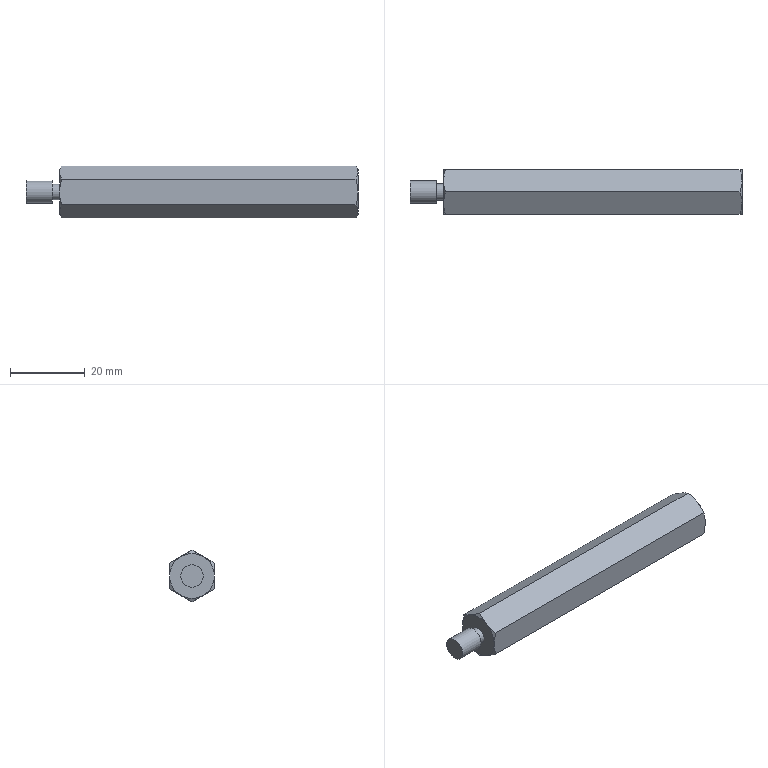Part | NX | features 5003_317_C-PLSBWRK12-80 2 | 1 solid | 26 faces | box 89 x 12 x 13.856 mm | volume 9868 mm3 | cone 13 | plane 10 | cylinder 3 | commonest cylinder face diameters 4.3 x1 4.917 x1 6 x1
STEP:
#1=CARTESIAN_POINT('',(218.525,69.,-97.));
#2=VERTEX_POINT('',#1);
#3=CARTESIAN_POINT('',(218.525,66.,-91.804));
#4=VERTEX_POINT('',#3);
#5=CARTESIAN_POINT('',(218.525,63.,-97.));
#6=DIRECTION('',(1.,0.,0.));
#7=DIRECTION('',(0.,1.,0.));
#8=AXIS2_PLACEMENT_3D('',#5,#6,#7);
#9=CIRCLE('',#8,6.);
#10=EDGE_CURVE('',#2,#4,#9,.T.);
#11=ORIENTED_EDGE('',*,*,#10,.F.);
#12=CARTESIAN_POINT('',(218.525,66.,-102.196));
#13=VERTEX_POINT('',#12);
#14=CARTESIAN_POINT('',(218.525,63.,-97.));
#15=DIRECTION('',(1.,0.,0.));
#16=DIRECTION('',(0.,1.,0.));
#17=AXIS2_PLACEMENT_3D('',#14,#15,#16);
#18=CIRCLE('',#17,6.);
#19=EDGE_CURVE('',#13,#2,#18,.T.);
#20=ORIENTED_EDGE('',*,*,#19,.F.);
#21=CARTESIAN_POINT('',(218.525,60.,-102.196));
#22=VERTEX_POINT('',#21);
#23=CARTESIAN_POINT('',(218.525,63.,-97.));
#24=DIRECTION('',(1.,0.,0.));
#25=DIRECTION('',(0.,1.,0.));
#26=AXIS2_PLACEMENT_3D('',#23,#24,#25);
#27=CIRCLE('',#26,6.);
#28=EDGE_CURVE('',#22,#13,#27,.T.);
#29=ORIENTED_EDGE('',*,*,#28,.F.);
#30=CARTESIAN_POINT('',(218.525,57.,-97.));
#31=VERTEX_POINT('',#30);
#32=CARTESIAN_POINT('',(218.525,63.,-97.));
#33=DIRECTION('',(1.,0.,0.));
#34=DIRECTION('',(0.,1.,0.));
#35=AXIS2_PLACEMENT_3D('',#32,#33,#34);
#36=CIRCLE('',#35,6.);
#37=EDGE_CURVE('',#31,#22,#36,.T.);
#38=ORIENTED_EDGE('',*,*,#37,.F.);
#39=CARTESIAN_POINT('',(218.525,60.,-91.804));
#40=VERTEX_POINT('',#39);
#41=CARTESIAN_POINT('',(218.525,63.,-97.));
#42=DIRECTION('',(-1.,0.,0.));
#43=DIRECTION('',(0.,-1.,0.));
#44=AXIS2_PLACEMENT_3D('',#41,#42,#43);
#45=CIRCLE('',#44,6.);
#46=EDGE_CURVE('',#31,#40,#45,.T.);
#47=ORIENTED_EDGE('',*,*,#46,.T.);
#48=CARTESIAN_POINT('',(218.525,63.,-97.));
#49=DIRECTION('',(1.,0.,0.));
#50=DIRECTION('',(0.,1.,0.));
#51=AXIS2_PLACEMENT_3D('',#48,#49,#50);
#52=CIRCLE('',#51,6.);
#53=EDGE_CURVE('',#4,#40,#52,.T.);
#54=ORIENTED_EDGE('',*,*,#53,.F.);
#55=EDGE_LOOP('',(#11,#20,#29,#38,#47,#54));
#56=FACE_BOUND('',#55,.T.);
#57=CARTESIAN_POINT('',(218.525,65.15,-97.));
#58=VERTEX_POINT('',#57);
#59=CARTESIAN_POINT('',(218.525,63.,-97.));
#60=DIRECTION('',(1.,0.,0.));
#61=DIRECTION('',(0.,1.,0.));
#62=AXIS2_PLACEMENT_3D('',#59,#60,#61);
#63=CIRCLE('',#62,2.15);
#64=EDGE_CURVE('',#58,#58,#63,.F.);
#65=ORIENTED_EDGE('',*,*,#64,.F.);
#66=EDGE_LOOP('',(#65));
#67=FACE_BOUND('',#66,.T.);
#68=CARTESIAN_POINT('',(218.525,63.,-97.));
#69=DIRECTION('',(1.,0.,0.));
#70=DIRECTION('',(0.,1.,0.));
#71=AXIS2_PLACEMENT_3D('',#68,#69,#70);
#72=PLANE('',#71);
#73=ADVANCED_FACE('',(#56,#67),#72,.F.);
#74=CARTESIAN_POINT('',(297.989,69.,-100.464));
#75=VERTEX_POINT('',#74);
#76=CARTESIAN_POINT('',(298.525,69.,-97.));
#77=VERTEX_POINT('',#76);
#78=CARTESIAN_POINT('',(297.989,69.,-100.464));
#79=CARTESIAN_POINT('',(298.314,69.,-99.337));
#80=CARTESIAN_POINT('',(298.525,69.,-98.171));
#81=CARTESIAN_POINT('',(298.525,69.,-97.));
#82=B_SPLINE_CURVE_WITH_KNOTS('',3,(#78,#79,#80,#81),.UNSPECIFIED.,.F.,.F.,(4,4),(0.00618,0.009685),.UNSPECIFIED.);
#83=EDGE_CURVE('',#75,#77,#82,.T.);
#84=ORIENTED_EDGE('',*,*,#83,.F.);
#85=CARTESIAN_POINT('',(219.061,69.,-100.464));
#86=VERTEX_POINT('',#85);
#87=CARTESIAN_POINT('',(298.525,69.,-100.464));
#88=DIRECTION('',(-1.,0.,0.));
#89=VECTOR('',#88,1000.);
#90=LINE('',#87,#89);
#91=EDGE_CURVE('',#75,#86,#90,.T.);
#92=ORIENTED_EDGE('',*,*,#91,.T.);
#93=CARTESIAN_POINT('',(219.061,69.,-100.464));
#94=CARTESIAN_POINT('',(218.736,69.,-99.337));
#95=CARTESIAN_POINT('',(218.525,69.,-98.171));
#96=CARTESIAN_POINT('',(218.525,69.,-97.));
#97=B_SPLINE_CURVE_WITH_KNOTS('',3,(#93,#94,#95,#96),.UNSPECIFIED.,.F.,.F.,(4,4),(0.00618,0.009685),.UNSPECIFIED.);
#98=EDGE_CURVE('',#2,#86,#97,.F.);
#99=ORIENTED_EDGE('',*,*,#98,.F.);
#100=CARTESIAN_POINT('',(219.061,69.,-93.536));
#101=VERTEX_POINT('',#100);
#102=CARTESIAN_POINT('',(218.525,69.,-97.));
#103=CARTESIAN_POINT('',(218.525,69.,-95.829));
#104=CARTESIAN_POINT('',(218.738,69.,-94.656));
#105=CARTESIAN_POINT('',(219.061,69.,-93.536));
#106=B_SPLINE_CURVE_WITH_KNOTS('',3,(#102,#103,#104,#105),.UNSPECIFIED.,.F.,.F.,(4,4),(0.009685,0.01319),.UNSPECIFIED.);
#107=EDGE_CURVE('',#101,#2,#106,.F.);
#108=ORIENTED_EDGE('',*,*,#107,.F.);
#109=CARTESIAN_POINT('',(297.989,69.,-93.536));
#110=VERTEX_POINT('',#109);
#111=CARTESIAN_POINT('',(298.525,69.,-93.536));
#112=DIRECTION('',(-1.,0.,0.));
#113=VECTOR('',#112,1000.);
#114=LINE('',#111,#113);
#115=EDGE_CURVE('',#110,#101,#114,.T.);
#116=ORIENTED_EDGE('',*,*,#115,.F.);
#117=CARTESIAN_POINT('',(298.525,69.,-97.));
#118=CARTESIAN_POINT('',(298.525,69.,-95.829));
#119=CARTESIAN_POINT('',(298.312,69.,-94.656));
#120=CARTESIAN_POINT('',(297.989,69.,-93.536));
#121=B_SPLINE_CURVE_WITH_KNOTS('',3,(#117,#118,#119,#120),.UNSPECIFIED.,.F.,.F.,(4,4),(0.009685,0.01319),.UNSPECIFIED.);
#122=EDGE_CURVE('',#77,#110,#121,.T.);
#123=ORIENTED_EDGE('',*,*,#122,.F.);
#124=EDGE_LOOP('',(#84,#92,#99,#108,#116,#123));
#125=FACE_BOUND('',#124,.T.);
#126=CARTESIAN_POINT('',(298.525,69.,-100.464));
#127=DIRECTION('',(0.,-1.,0.));
#128=DIRECTION('',(0.,0.,-1.));
#129=AXIS2_PLACEMENT_3D('',#126,#127,#128);
#130=PLANE('',#129);
#131=ADVANCED_FACE('',(#125),#130,.F.);
#132=CARTESIAN_POINT('',(298.525,66.,-91.804));
#133=VERTEX_POINT('',#132);
#134=CARTESIAN_POINT('',(297.989,69.,-93.536));
#135=CARTESIAN_POINT('',(298.316,68.018,-92.969));
#136=CARTESIAN_POINT('',(298.525,67.022,-92.394));
#137=CARTESIAN_POINT('',(298.525,66.,-91.804));
#138=B_SPLINE_CURVE_WITH_KNOTS('',3,(#134,#135,#136,#137),.UNSPECIFIED.,.F.,.F.,(4,4),(0.000000238,0.003505),.UNSPECIFIED.);
#139=EDGE_CURVE('',#110,#133,#138,.T.);
#140=ORIENTED_EDGE('',*,*,#139,.F.);
#141=ORIENTED_EDGE('',*,*,#115,.T.);
#142=CARTESIAN_POINT('',(218.525,66.,-91.804));
#143=CARTESIAN_POINT('',(218.525,67.018,-92.392));
#144=CARTESIAN_POINT('',(218.735,68.021,-92.971));
#145=CARTESIAN_POINT('',(219.061,69.,-93.536));
#146=B_SPLINE_CURVE_WITH_KNOTS('',3,(#142,#143,#144,#145),.UNSPECIFIED.,.F.,.F.,(4,4),(0.003505,0.006997),.UNSPECIFIED.);
#147=EDGE_CURVE('',#4,#101,#146,.T.);
#148=ORIENTED_EDGE('',*,*,#147,.F.);
#149=CARTESIAN_POINT('',(219.061,63.,-90.072));
#150=VERTEX_POINT('',#149);
#151=CARTESIAN_POINT('',(219.061,63.,-90.072));
#152=CARTESIAN_POINT('',(218.734,63.982,-90.638));
#153=CARTESIAN_POINT('',(218.525,64.978,-91.214));
#154=CARTESIAN_POINT('',(218.525,66.,-91.804));
#155=B_SPLINE_CURVE_WITH_KNOTS('',3,(#151,#152,#153,#154),.UNSPECIFIED.,.F.,.F.,(4,4),(0.000000238,0.003505),.UNSPECIFIED.);
#156=EDGE_CURVE('',#150,#4,#155,.T.);
#157=ORIENTED_EDGE('',*,*,#156,.F.);
#158=CARTESIAN_POINT('',(297.989,63.,-90.072));
#159=VERTEX_POINT('',#158);
#160=CARTESIAN_POINT('',(298.525,63.,-90.072));
#161=DIRECTION('',(-1.,0.,0.));
#162=VECTOR('',#161,1000.);
#163=LINE('',#160,#162);
#164=EDGE_CURVE('',#159,#150,#163,.T.);
#165=ORIENTED_EDGE('',*,*,#164,.F.);
#166=CARTESIAN_POINT('',(298.525,66.,-91.804));
#167=CARTESIAN_POINT('',(298.525,64.982,-91.216));
#168=CARTESIAN_POINT('',(298.315,63.979,-90.637));
#169=CARTESIAN_POINT('',(297.989,63.,-90.072));
#170=B_SPLINE_CURVE_WITH_KNOTS('',3,(#166,#167,#168,#169),.UNSPECIFIED.,.F.,.F.,(4,4),(0.003505,0.006997),.UNSPECIFIED.);
#171=EDGE_CURVE('',#133,#159,#170,.T.);
#172=ORIENTED_EDGE('',*,*,#171,.F.);
#173=EDGE_LOOP('',(#140,#141,#148,#157,#165,#172));
#174=FACE_BOUND('',#173,.T.);
#175=CARTESIAN_POINT('',(298.525,69.,-93.536));
#176=DIRECTION('',(0.,-0.5,-0.866));
#177=DIRECTION('',(0.,0.866,-0.5));
#178=AXIS2_PLACEMENT_3D('',#175,#176,#177);
#179=PLANE('',#178);
#180=ADVANCED_FACE('',(#174),#179,.F.);
#181=CARTESIAN_POINT('',(298.525,60.,-91.804));
#182=VERTEX_POINT('',#181);
#183=CARTESIAN_POINT('',(297.989,63.,-90.072));
#184=CARTESIAN_POINT('',(298.316,62.018,-90.638));
#185=CARTESIAN_POINT('',(298.525,61.022,-91.214));
#186=CARTESIAN_POINT('',(298.525,60.,-91.804));
#187=B_SPLINE_CURVE_WITH_KNOTS('',3,(#183,#184,#185,#186),.UNSPECIFIED.,.F.,.F.,(4,4),(0.000000238,0.003505),.UNSPECIFIED.);
#188=EDGE_CURVE('',#159,#182,#187,.T.);
#189=ORIENTED_EDGE('',*,*,#188,.F.);
#190=ORIENTED_EDGE('',*,*,#164,.T.);
#191=CARTESIAN_POINT('',(218.525,60.,-91.804));
#192=CARTESIAN_POINT('',(218.525,61.018,-91.216));
#193=CARTESIAN_POINT('',(218.735,62.021,-90.637));
#194=CARTESIAN_POINT('',(219.061,63.,-90.072));
#195=B_SPLINE_CURVE_WITH_KNOTS('',3,(#191,#192,#193,#194),.UNSPECIFIED.,.F.,.F.,(4,4),(0.003505,0.006997),.UNSPECIFIED.);
#196=EDGE_CURVE('',#40,#150,#195,.T.);
#197=ORIENTED_EDGE('',*,*,#196,.F.);
#198=CARTESIAN_POINT('',(219.061,57.,-93.536));
#199=VERTEX_POINT('',#198);
#200=CARTESIAN_POINT('',(219.061,57.,-93.536));
#201=CARTESIAN_POINT('',(218.734,57.982,-92.969));
#202=CARTESIAN_POINT('',(218.525,58.978,-92.394));
#203=CARTESIAN_POINT('',(218.525,60.,-91.804));
#204=B_SPLINE_CURVE_WITH_KNOTS('',3,(#200,#201,#202,#203),.UNSPECIFIED.,.F.,.F.,(4,4),(0.000000238,0.003505),.UNSPECIFIED.);
#205=EDGE_CURVE('',#199,#40,#204,.T.);
#206=ORIENTED_EDGE('',*,*,#205,.F.);
#207=CARTESIAN_POINT('',(297.989,57.,-93.536));
#208=VERTEX_POINT('',#207);
#209=CARTESIAN_POINT('',(298.525,57.,-93.536));
#210=DIRECTION('',(-1.,0.,0.));
#211=VECTOR('',#210,1000.);
#212=LINE('',#209,#211);
#213=EDGE_CURVE('',#208,#199,#212,.T.);
#214=ORIENTED_EDGE('',*,*,#213,.F.);
#215=CARTESIAN_POINT('',(298.525,60.,-91.804));
#216=CARTESIAN_POINT('',(298.525,58.982,-92.392));
#217=CARTESIAN_POINT('',(298.315,57.979,-92.971));
#218=CARTESIAN_POINT('',(297.989,57.,-93.536));
#219=B_SPLINE_CURVE_WITH_KNOTS('',3,(#215,#216,#217,#218),.UNSPECIFIED.,.F.,.F.,(4,4),(0.003505,0.006997),.UNSPECIFIED.);
#220=EDGE_CURVE('',#182,#208,#219,.T.);
#221=ORIENTED_EDGE('',*,*,#220,.F.);
#222=EDGE_LOOP('',(#189,#190,#197,#206,#214,#221));
#223=FACE_BOUND('',#222,.T.);
#224=CARTESIAN_POINT('',(298.525,63.,-90.072));
#225=DIRECTION('',(0.,0.5,-0.866));
#226=DIRECTION('',(0.,0.866,0.5));
#227=AXIS2_PLACEMENT_3D('',#224,#225,#226);
#228=PLANE('',#227);
#229=ADVANCED_FACE('',(#223),#228,.F.);
#230=CARTESIAN_POINT('',(298.525,57.,-97.));
#231=VERTEX_POINT('',#230);
#232=CARTESIAN_POINT('',(298.525,57.,-97.));
#233=CARTESIAN_POINT('',(298.525,57.,-95.829));
#234=CARTESIAN_POINT('',(298.312,57.,-94.656));
#235=CARTESIAN_POINT('',(297.989,57.,-93.536));
#236=B_SPLINE_CURVE_WITH_KNOTS('',3,(#232,#233,#234,#235),.UNSPECIFIED.,.F.,.F.,(4,4),(0.009685,0.01319),.UNSPECIFIED.);
#237=EDGE_CURVE('',#208,#231,#236,.F.);
#238=ORIENTED_EDGE('',*,*,#237,.F.);
#239=ORIENTED_EDGE('',*,*,#213,.T.);
#240=CARTESIAN_POINT('',(218.525,57.,-97.));
#241=CARTESIAN_POINT('',(218.525,57.,-95.829));
#242=CARTESIAN_POINT('',(218.738,57.,-94.656));
#243=CARTESIAN_POINT('',(219.061,57.,-93.536));
#244=B_SPLINE_CURVE_WITH_KNOTS('',3,(#240,#241,#242,#243),.UNSPECIFIED.,.F.,.F.,(4,4),(0.009685,0.01319),.UNSPECIFIED.);
#245=EDGE_CURVE('',#31,#199,#244,.T.);
#246=ORIENTED_EDGE('',*,*,#245,.F.);
#247=CARTESIAN_POINT('',(219.061,57.,-100.464));
#248=VERTEX_POINT('',#247);
#249=CARTESIAN_POINT('',(219.061,57.,-100.464));
#250=CARTESIAN_POINT('',(218.736,57.,-99.337));
#251=CARTESIAN_POINT('',(218.525,57.,-98.171));
#252=CARTESIAN_POINT('',(218.525,57.,-97.));
#253=B_SPLINE_CURVE_WITH_KNOTS('',3,(#249,#250,#251,#252),.UNSPECIFIED.,.F.,.F.,(4,4),(0.00618,0.009685),.UNSPECIFIED.);
#254=EDGE_CURVE('',#248,#31,#253,.T.);
#255=ORIENTED_EDGE('',*,*,#254,.F.);
#256=CARTESIAN_POINT('',(297.989,57.,-100.464));
#257=VERTEX_POINT('',#256);
#258=CARTESIAN_POINT('',(298.525,57.,-100.464));
#259=DIRECTION('',(-1.,0.,0.));
#260=VECTOR('',#259,1000.);
#261=LINE('',#258,#260);
#262=EDGE_CURVE('',#257,#248,#261,.T.);
#263=ORIENTED_EDGE('',*,*,#262,.F.);
#264=CARTESIAN_POINT('',(297.989,57.,-100.464));
#265=CARTESIAN_POINT('',(298.314,57.,-99.337));
#266=CARTESIAN_POINT('',(298.525,57.,-98.171));
#267=CARTESIAN_POINT('',(298.525,57.,-97.));
#268=B_SPLINE_CURVE_WITH_KNOTS('',3,(#264,#265,#266,#267),.UNSPECIFIED.,.F.,.F.,(4,4),(0.00618,0.009685),.UNSPECIFIED.);
#269=EDGE_CURVE('',#231,#257,#268,.F.);
#270=ORIENTED_EDGE('',*,*,#269,.F.);
#271=EDGE_LOOP('',(#238,#239,#246,#255,#263,#270));
#272=FACE_BOUND('',#271,.T.);
#273=CARTESIAN_POINT('',(298.525,57.,-93.536));
#274=DIRECTION('',(0.,1.,0.));
#275=DIRECTION('',(-1.,0.,0.));
#276=AXIS2_PLACEMENT_3D('',#273,#274,#275);
#277=PLANE('',#276);
#278=ADVANCED_FACE('',(#272),#277,.F.);
#279=CARTESIAN_POINT('',(298.525,60.,-102.196));
#280=VERTEX_POINT('',#279);
#281=CARTESIAN_POINT('',(297.989,57.,-100.464));
#282=CARTESIAN_POINT('',(298.316,57.982,-101.031));
#283=CARTESIAN_POINT('',(298.525,58.978,-101.606));
#284=CARTESIAN_POINT('',(298.525,60.,-102.196));
#285=B_SPLINE_CURVE_WITH_KNOTS('',3,(#281,#282,#283,#284),.UNSPECIFIED.,.F.,.F.,(4,4),(0.000000238,0.003505),.UNSPECIFIED.);
#286=EDGE_CURVE('',#257,#280,#285,.T.);
#287=ORIENTED_EDGE('',*,*,#286,.F.);
#288=ORIENTED_EDGE('',*,*,#262,.T.);
#289=CARTESIAN_POINT('',(218.525,60.,-102.196));
#290=CARTESIAN_POINT('',(218.525,58.982,-101.608));
#291=CARTESIAN_POINT('',(218.735,57.979,-101.029));
#292=CARTESIAN_POINT('',(219.061,57.,-100.464));
#293=B_SPLINE_CURVE_WITH_KNOTS('',3,(#289,#290,#291,#292),.UNSPECIFIED.,.F.,.F.,(4,4),(0.003505,0.006997),.UNSPECIFIED.);
#294=EDGE_CURVE('',#22,#248,#293,.T.);
#295=ORIENTED_EDGE('',*,*,#294,.F.);
#296=CARTESIAN_POINT('',(219.061,63.,-103.928));
#297=VERTEX_POINT('',#296);
#298=CARTESIAN_POINT('',(219.061,63.,-103.928));
#299=CARTESIAN_POINT('',(218.734,62.018,-103.362));
#300=CARTESIAN_POINT('',(218.525,61.022,-102.786));
#301=CARTESIAN_POINT('',(218.525,60.,-102.196));
#302=B_SPLINE_CURVE_WITH_KNOTS('',3,(#298,#299,#300,#301),.UNSPECIFIED.,.F.,.F.,(4,4),(0.000000238,0.003505),.UNSPECIFIED.);
#303=EDGE_CURVE('',#297,#22,#302,.T.);
#304=ORIENTED_EDGE('',*,*,#303,.F.);
#305=CARTESIAN_POINT('',(297.989,63.,-103.928));
#306=VERTEX_POINT('',#305);
#307=CARTESIAN_POINT('',(298.525,63.,-103.928));
#308=DIRECTION('',(-1.,0.,0.));
#309=VECTOR('',#308,1000.);
#310=LINE('',#307,#309);
#311=EDGE_CURVE('',#306,#297,#310,.T.);
#312=ORIENTED_EDGE('',*,*,#311,.F.);
#313=CARTESIAN_POINT('',(298.525,60.,-102.196));
#314=CARTESIAN_POINT('',(298.525,61.018,-102.784));
#315=CARTESIAN_POINT('',(298.315,62.021,-103.363));
#316=CARTESIAN_POINT('',(297.989,63.,-103.928));
#317=B_SPLINE_CURVE_WITH_KNOTS('',3,(#313,#314,#315,#316),.UNSPECIFIED.,.F.,.F.,(4,4),(0.003505,0.006997),.UNSPECIFIED.);
#318=EDGE_CURVE('',#280,#306,#317,.T.);
#319=ORIENTED_EDGE('',*,*,#318,.F.);
#320=EDGE_LOOP('',(#287,#288,#295,#304,#312,#319));
#321=FACE_BOUND('',#320,.T.);
#322=CARTESIAN_POINT('',(298.525,57.,-100.464));
#323=DIRECTION('',(0.,0.5,0.866));
#324=DIRECTION('',(0.,-0.866,0.5));
#325=AXIS2_PLACEMENT_3D('',#322,#323,#324);
#326=PLANE('',#325);
#327=ADVANCED_FACE('',(#321),#326,.F.);
#328=CARTESIAN_POINT('',(298.525,66.,-102.196));
#329=VERTEX_POINT('',#328);
#330=CARTESIAN_POINT('',(297.989,63.,-103.928));
#331=CARTESIAN_POINT('',(298.316,63.982,-103.362));
#332=CARTESIAN_POINT('',(298.525,64.978,-102.786));
#333=CARTESIAN_POINT('',(298.525,66.,-102.196));
#334=B_SPLINE_CURVE_WITH_KNOTS('',3,(#330,#331,#332,#333),.UNSPECIFIED.,.F.,.F.,(4,4),(0.000000238,0.003505),.UNSPECIFIED.);
#335=EDGE_CURVE('',#306,#329,#334,.T.);
#336=ORIENTED_EDGE('',*,*,#335,.F.);
#337=ORIENTED_EDGE('',*,*,#311,.T.);
#338=CARTESIAN_POINT('',(218.525,66.,-102.196));
#339=CARTESIAN_POINT('',(218.525,64.982,-102.784));
#340=CARTESIAN_POINT('',(218.735,63.979,-103.363));
#341=CARTESIAN_POINT('',(219.061,63.,-103.928));
#342=B_SPLINE_CURVE_WITH_KNOTS('',3,(#338,#339,#340,#341),.UNSPECIFIED.,.F.,.F.,(4,4),(0.003505,0.006997),.UNSPECIFIED.);
#343=EDGE_CURVE('',#13,#297,#342,.T.);
#344=ORIENTED_EDGE('',*,*,#343,.F.);
#345=CARTESIAN_POINT('',(219.061,69.,-100.464));
#346=CARTESIAN_POINT('',(218.734,68.018,-101.031));
#347=CARTESIAN_POINT('',(218.525,67.022,-101.606));
#348=CARTESIAN_POINT('',(218.525,66.,-102.196));
#349=B_SPLINE_CURVE_WITH_KNOTS('',3,(#345,#346,#347,#348),.UNSPECIFIED.,.F.,.F.,(4,4),(0.000000238,0.003505),.UNSPECIFIED.);
#350=EDGE_CURVE('',#86,#13,#349,.T.);
#351=ORIENTED_EDGE('',*,*,#350,.F.);
#352=ORIENTED_EDGE('',*,*,#91,.F.);
#353=CARTESIAN_POINT('',(298.525,66.,-102.196));
#354=CARTESIAN_POINT('',(298.525,67.018,-101.608));
#355=CARTESIAN_POINT('',(298.315,68.021,-101.029));
#356=CARTESIAN_POINT('',(297.989,69.,-100.464));
#357=B_SPLINE_CURVE_WITH_KNOTS('',3,(#353,#354,#355,#356),.UNSPECIFIED.,.F.,.F.,(4,4),(0.003505,0.006997),.UNSPECIFIED.);
#358=EDGE_CURVE('',#329,#75,#357,.T.);
#359=ORIENTED_EDGE('',*,*,#358,.F.);
#360=EDGE_LOOP('',(#336,#337,#344,#351,#352,#359));
#361=FACE_BOUND('',#360,.T.);
#362=CARTESIAN_POINT('',(298.525,63.,-103.928));
#363=DIRECTION('',(0.,-0.5,0.866));
#364=DIRECTION('',(0.,-0.866,-0.5));
#365=AXIS2_PLACEMENT_3D('',#362,#363,#364);
#366=PLANE('',#365);
#367=ADVANCED_FACE('',(#361),#366,.F.);
#368=ORIENTED_EDGE('',*,*,#98,.T.);
#369=ORIENTED_EDGE('',*,*,#350,.T.);
#370=ORIENTED_EDGE('',*,*,#19,.T.);
#371=EDGE_LOOP('',(#368,#369,#370));
#372=FACE_BOUND('',#371,.T.);
#373=CARTESIAN_POINT('',(218.525,63.,-97.));
#374=DIRECTION('',(1.,0.,0.));
#375=DIRECTION('',(0.,1.,0.));
#376=AXIS2_PLACEMENT_3D('',#373,#374,#375);
#377=CONICAL_SURFACE('',#376,6.,1.047);
#378=ADVANCED_FACE('',(#372),#377,.T.);
#379=ORIENTED_EDGE('',*,*,#303,.T.);
#380=ORIENTED_EDGE('',*,*,#28,.T.);
#381=ORIENTED_EDGE('',*,*,#343,.T.);
#382=EDGE_LOOP('',(#379,#380,#381));
#383=FACE_BOUND('',#382,.T.);
#384=CARTESIAN_POINT('',(218.525,63.,-97.));
#385=DIRECTION('',(1.,0.,0.));
#386=DIRECTION('',(0.,1.,0.));
#387=AXIS2_PLACEMENT_3D('',#384,#385,#386);
#388=CONICAL_SURFACE('',#387,6.,1.047);
#389=ADVANCED_FACE('',(#383),#388,.T.);
#390=ORIENTED_EDGE('',*,*,#254,.T.);
#391=ORIENTED_EDGE('',*,*,#37,.T.);
#392=ORIENTED_EDGE('',*,*,#294,.T.);
#393=EDGE_LOOP('',(#390,#391,#392));
#394=FACE_BOUND('',#393,.T.);
#395=CARTESIAN_POINT('',(218.525,63.,-97.));
#396=DIRECTION('',(1.,0.,0.));
#397=DIRECTION('',(0.,1.,0.));
#398=AXIS2_PLACEMENT_3D('',#395,#396,#397);
#399=CONICAL_SURFACE('',#398,6.,1.047);
#400=ADVANCED_FACE('',(#394),#399,.T.);
#401=ORIENTED_EDGE('',*,*,#205,.T.);
#402=ORIENTED_EDGE('',*,*,#46,.F.);
#403=ORIENTED_EDGE('',*,*,#245,.T.);
#404=EDGE_LOOP('',(#401,#402,#403));
#405=FACE_BOUND('',#404,.T.);
#406=CARTESIAN_POINT('',(218.525,63.,-97.));
#407=DIRECTION('',(1.,0.,0.));
#408=DIRECTION('',(0.,1.,0.));
#409=AXIS2_PLACEMENT_3D('',#406,#407,#408);
#410=CONICAL_SURFACE('',#409,6.,1.047);
#411=ADVANCED_FACE('',(#405),#410,.T.);
#412=ORIENTED_EDGE('',*,*,#196,.T.);
#413=ORIENTED_EDGE('',*,*,#156,.T.);
#414=ORIENTED_EDGE('',*,*,#53,.T.);
#415=EDGE_LOOP('',(#412,#413,#414));
#416=FACE_BOUND('',#415,.T.);
#417=CARTESIAN_POINT('',(218.525,63.,-97.));
#418=DIRECTION('',(1.,0.,0.));
#419=DIRECTION('',(0.,1.,0.));
#420=AXIS2_PLACEMENT_3D('',#417,#418,#419);
#421=CONICAL_SURFACE('',#420,6.,1.047);
#422=ADVANCED_FACE('',(#416),#421,.T.);
#423=ORIENTED_EDGE('',*,*,#147,.T.);
#424=ORIENTED_EDGE('',*,*,#107,.T.);
#425=ORIENTED_EDGE('',*,*,#10,.T.);
#426=EDGE_LOOP('',(#423,#424,#425));
#427=FACE_BOUND('',#426,.T.);
#428=CARTESIAN_POINT('',(218.525,63.,-97.));
#429=DIRECTION('',(1.,0.,0.));
#430=DIRECTION('',(0.,1.,0.));
#431=AXIS2_PLACEMENT_3D('',#428,#429,#430);
#432=CONICAL_SURFACE('',#431,6.,1.047);
#433=ADVANCED_FACE('',(#427),#432,.T.);
#434=ORIENTED_EDGE('',*,*,#83,.T.);
#435=CARTESIAN_POINT('',(298.525,63.,-97.));
#436=DIRECTION('',(1.,0.,0.));
#437=DIRECTION('',(0.,1.,0.));
#438=AXIS2_PLACEMENT_3D('',#435,#436,#437);
#439=CIRCLE('',#438,6.);
#440=EDGE_CURVE('',#329,#77,#439,.T.);
#441=ORIENTED_EDGE('',*,*,#440,.F.);
#442=ORIENTED_EDGE('',*,*,#358,.T.);
#443=EDGE_LOOP('',(#434,#441,#442));
#444=FACE_BOUND('',#443,.T.);
#445=CARTESIAN_POINT('',(297.989,63.,-97.));
#446=DIRECTION('',(-1.,0.,0.));
#447=DIRECTION('',(0.,-1.,0.));
#448=AXIS2_PLACEMENT_3D('',#445,#446,#447);
#449=CONICAL_SURFACE('',#448,6.928,1.047);
#450=ADVANCED_FACE('',(#444),#449,.T.);
#451=ORIENTED_EDGE('',*,*,#318,.T.);
#452=ORIENTED_EDGE('',*,*,#335,.T.);
#453=CARTESIAN_POINT('',(298.525,63.,-97.));
#454=DIRECTION('',(1.,0.,0.));
#455=DIRECTION('',(0.,1.,0.));
#456=AXIS2_PLACEMENT_3D('',#453,#454,#455);
#457=CIRCLE('',#456,6.);
#458=EDGE_CURVE('',#280,#329,#457,.T.);
#459=ORIENTED_EDGE('',*,*,#458,.F.);
#460=EDGE_LOOP('',(#451,#452,#459));
#461=FACE_BOUND('',#460,.T.);
#462=CARTESIAN_POINT('',(297.989,63.,-97.));
#463=DIRECTION('',(-1.,0.,0.));
#464=DIRECTION('',(0.,-1.,0.));
#465=AXIS2_PLACEMENT_3D('',#462,#463,#464);
#466=CONICAL_SURFACE('',#465,6.928,1.047);
#467=ADVANCED_FACE('',(#461),#466,.T.);
#468=ORIENTED_EDGE('',*,*,#269,.T.);
#469=ORIENTED_EDGE('',*,*,#286,.T.);
#470=CARTESIAN_POINT('',(298.525,63.,-97.));
#471=DIRECTION('',(1.,0.,0.));
#472=DIRECTION('',(0.,1.,0.));
#473=AXIS2_PLACEMENT_3D('',#470,#471,#472);
#474=CIRCLE('',#473,6.);
#475=EDGE_CURVE('',#231,#280,#474,.T.);
#476=ORIENTED_EDGE('',*,*,#475,.F.);
#477=EDGE_LOOP('',(#468,#469,#476));
#478=FACE_BOUND('',#477,.T.);
#479=CARTESIAN_POINT('',(297.989,63.,-97.));
#480=DIRECTION('',(-1.,0.,0.));
#481=DIRECTION('',(0.,-1.,0.));
#482=AXIS2_PLACEMENT_3D('',#479,#480,#481);
#483=CONICAL_SURFACE('',#482,6.928,1.047);
#484=ADVANCED_FACE('',(#478),#483,.T.);
#485=ORIENTED_EDGE('',*,*,#220,.T.);
#486=ORIENTED_EDGE('',*,*,#237,.T.);
#487=CARTESIAN_POINT('',(298.525,63.,-97.));
#488=DIRECTION('',(-1.,0.,0.));
#489=DIRECTION('',(0.,-1.,0.));
#490=AXIS2_PLACEMENT_3D('',#487,#488,#489);
#491=CIRCLE('',#490,6.);
#492=EDGE_CURVE('',#231,#182,#491,.T.);
#493=ORIENTED_EDGE('',*,*,#492,.T.);
#494=EDGE_LOOP('',(#485,#486,#493));
#495=FACE_BOUND('',#494,.T.);
#496=CARTESIAN_POINT('',(297.989,63.,-97.));
#497=DIRECTION('',(-1.,0.,0.));
#498=DIRECTION('',(0.,-1.,0.));
#499=AXIS2_PLACEMENT_3D('',#496,#497,#498);
#500=CONICAL_SURFACE('',#499,6.928,1.047);
#501=ADVANCED_FACE('',(#495),#500,.T.);
#502=ORIENTED_EDGE('',*,*,#171,.T.);
#503=ORIENTED_EDGE('',*,*,#188,.T.);
#504=CARTESIAN_POINT('',(298.525,63.,-97.));
#505=DIRECTION('',(1.,0.,0.));
#506=DIRECTION('',(0.,1.,0.));
#507=AXIS2_PLACEMENT_3D('',#504,#505,#506);
#508=CIRCLE('',#507,6.);
#509=EDGE_CURVE('',#133,#182,#508,.T.);
#510=ORIENTED_EDGE('',*,*,#509,.F.);
#511=EDGE_LOOP('',(#502,#503,#510));
#512=FACE_BOUND('',#511,.T.);
#513=CARTESIAN_POINT('',(297.989,63.,-97.));
#514=DIRECTION('',(-1.,0.,0.));
#515=DIRECTION('',(0.,-1.,0.));
#516=AXIS2_PLACEMENT_3D('',#513,#514,#515);
#517=CONICAL_SURFACE('',#516,6.928,1.047);
#518=ADVANCED_FACE('',(#512),#517,.T.);
#519=ORIENTED_EDGE('',*,*,#122,.T.);
#520=ORIENTED_EDGE('',*,*,#139,.T.);
#521=CARTESIAN_POINT('',(298.525,63.,-97.));
#522=DIRECTION('',(1.,0.,0.));
#523=DIRECTION('',(0.,1.,0.));
#524=AXIS2_PLACEMENT_3D('',#521,#522,#523);
#525=CIRCLE('',#524,6.);
#526=EDGE_CURVE('',#77,#133,#525,.T.);
#527=ORIENTED_EDGE('',*,*,#526,.F.);
#528=EDGE_LOOP('',(#519,#520,#527));
#529=FACE_BOUND('',#528,.T.);
#530=CARTESIAN_POINT('',(297.989,63.,-97.));
#531=DIRECTION('',(-1.,0.,0.));
#532=DIRECTION('',(0.,-1.,0.));
#533=AXIS2_PLACEMENT_3D('',#530,#531,#532);
#534=CONICAL_SURFACE('',#533,6.928,1.047);
#535=ADVANCED_FACE('',(#529),#534,.T.);
#536=CARTESIAN_POINT('',(298.525,65.459,-97.));
#537=VERTEX_POINT('',#536);
#538=CARTESIAN_POINT('',(298.525,63.,-97.));
#539=DIRECTION('',(1.,0.,0.));
#540=DIRECTION('',(0.,1.,0.));
#541=AXIS2_PLACEMENT_3D('',#538,#539,#540);
#542=CIRCLE('',#541,2.458);
#543=EDGE_CURVE('',#537,#537,#542,.T.);
#544=ORIENTED_EDGE('',*,*,#543,.F.);
#545=EDGE_LOOP('',(#544));
#546=FACE_BOUND('',#545,.T.);
#547=ORIENTED_EDGE('',*,*,#440,.T.);
#548=ORIENTED_EDGE('',*,*,#526,.T.);
#549=ORIENTED_EDGE('',*,*,#509,.T.);
#550=ORIENTED_EDGE('',*,*,#492,.F.);
#551=ORIENTED_EDGE('',*,*,#475,.T.);
#552=ORIENTED_EDGE('',*,*,#458,.T.);
#553=EDGE_LOOP('',(#547,#548,#549,#550,#551,#552));
#554=FACE_BOUND('',#553,.T.);
#555=CARTESIAN_POINT('',(298.525,63.,-97.));
#556=DIRECTION('',(1.,0.,0.));
#557=DIRECTION('',(0.,1.,0.));
#558=AXIS2_PLACEMENT_3D('',#555,#556,#557);
#559=PLANE('',#558);
#560=ADVANCED_FACE('',(#546,#554),#559,.T.);
#561=CARTESIAN_POINT('',(280.048,63.,-97.));
#562=VERTEX_POINT('',#561);
#563=VERTEX_LOOP('',#562);
#564=FACE_BOUND('',#563,.T.);
#565=CARTESIAN_POINT('',(281.525,65.459,-97.));
#566=VERTEX_POINT('',#565);
#567=CARTESIAN_POINT('',(281.525,63.,-97.));
#568=DIRECTION('',(1.,0.,0.));
#569=DIRECTION('',(0.,1.,0.));
#570=AXIS2_PLACEMENT_3D('',#567,#568,#569);
#571=CIRCLE('',#570,2.458);
#572=EDGE_CURVE('',#566,#566,#571,.T.);
#573=ORIENTED_EDGE('',*,*,#572,.T.);
#574=EDGE_LOOP('',(#573));
#575=FACE_BOUND('',#574,.T.);
#576=CARTESIAN_POINT('',(281.525,63.,-97.));
#577=DIRECTION('',(1.,0.,0.));
#578=DIRECTION('',(0.,1.,0.));
#579=AXIS2_PLACEMENT_3D('',#576,#577,#578);
#580=CONICAL_SURFACE('',#579,2.458,1.03);
#581=ADVANCED_FACE('',(#564,#575),#580,.F.);
#582=ORIENTED_EDGE('',*,*,#572,.F.);
#583=EDGE_LOOP('',(#582));
#584=FACE_BOUND('',#583,.T.);
#585=ORIENTED_EDGE('',*,*,#543,.T.);
#586=EDGE_LOOP('',(#585));
#587=FACE_BOUND('',#586,.T.);
#588=CARTESIAN_POINT('',(298.525,63.,-97.));
#589=DIRECTION('',(1.,0.,0.));
#590=DIRECTION('',(0.,1.,0.));
#591=AXIS2_PLACEMENT_3D('',#588,#589,#590);
#592=CYLINDRICAL_SURFACE('',#591,2.458);
#593=ADVANCED_FACE('',(#584,#587),#592,.F.);
#594=CARTESIAN_POINT('',(216.525,60.85,-97.));
#595=VERTEX_POINT('',#594);
#596=CARTESIAN_POINT('',(216.525,63.,-97.));
#597=DIRECTION('',(-1.,0.,0.));
#598=DIRECTION('',(0.,-1.,0.));
#599=AXIS2_PLACEMENT_3D('',#596,#597,#598);
#600=CIRCLE('',#599,2.15);
#601=EDGE_CURVE('',#595,#595,#600,.T.);
#602=ORIENTED_EDGE('',*,*,#601,.F.);
#603=EDGE_LOOP('',(#602));
#604=FACE_BOUND('',#603,.T.);
#605=ORIENTED_EDGE('',*,*,#64,.T.);
#606=EDGE_LOOP('',(#605));
#607=FACE_BOUND('',#606,.T.);
#608=CARTESIAN_POINT('',(205.075,63.,-97.));
#609=DIRECTION('',(-1.,0.,0.));
#610=DIRECTION('',(0.,-1.,0.));
#611=AXIS2_PLACEMENT_3D('',#608,#609,#610);
#612=CYLINDRICAL_SURFACE('',#611,2.15);
#613=ADVANCED_FACE('',(#604,#607),#612,.T.);
#614=CARTESIAN_POINT('',(216.525,60.,-97.));
#615=VERTEX_POINT('',#614);
#616=CARTESIAN_POINT('',(216.525,63.,-97.));
#617=DIRECTION('',(-1.,0.,0.));
#618=DIRECTION('',(0.,-1.,0.));
#619=AXIS2_PLACEMENT_3D('',#616,#617,#618);
#620=CIRCLE('',#619,3.);
#621=EDGE_CURVE('',#615,#615,#620,.T.);
#622=ORIENTED_EDGE('',*,*,#621,.F.);
#623=EDGE_LOOP('',(#622));
#624=FACE_BOUND('',#623,.T.);
#625=ORIENTED_EDGE('',*,*,#601,.T.);
#626=EDGE_LOOP('',(#625));
#627=FACE_BOUND('',#626,.T.);
#628=CARTESIAN_POINT('',(216.525,63.,-94.85));
#629=DIRECTION('',(-1.,0.,0.));
#630=DIRECTION('',(0.,-1.,0.));
#631=AXIS2_PLACEMENT_3D('',#628,#629,#630);
#632=PLANE('',#631);
#633=ADVANCED_FACE('',(#624,#627),#632,.F.);
#634=CARTESIAN_POINT('',(209.525,60.,-97.));
#635=VERTEX_POINT('',#634);
#636=CARTESIAN_POINT('',(209.525,63.,-97.));
#637=DIRECTION('',(-1.,0.,0.));
#638=DIRECTION('',(0.,-1.,0.));
#639=AXIS2_PLACEMENT_3D('',#636,#637,#638);
#640=CIRCLE('',#639,3.);
#641=EDGE_CURVE('',#635,#635,#640,.T.);
#642=ORIENTED_EDGE('',*,*,#641,.F.);
#643=EDGE_LOOP('',(#642));
#644=FACE_BOUND('',#643,.T.);
#645=ORIENTED_EDGE('',*,*,#621,.T.);
#646=EDGE_LOOP('',(#645));
#647=FACE_BOUND('',#646,.T.);
#648=CARTESIAN_POINT('',(205.075,63.,-97.));
#649=DIRECTION('',(-1.,0.,0.));
#650=DIRECTION('',(0.,-1.,0.));
#651=AXIS2_PLACEMENT_3D('',#648,#649,#650);
#652=CYLINDRICAL_SURFACE('',#651,3.);
#653=ADVANCED_FACE('',(#644,#647),#652,.T.);
#654=ORIENTED_EDGE('',*,*,#641,.T.);
#655=EDGE_LOOP('',(#654));
#656=FACE_BOUND('',#655,.T.);
#657=CARTESIAN_POINT('',(209.525,63.,-94.));
#658=DIRECTION('',(1.,0.,0.));
#659=DIRECTION('',(0.,1.,0.));
#660=AXIS2_PLACEMENT_3D('',#657,#658,#659);
#661=PLANE('',#660);
#662=ADVANCED_FACE('',(#656),#661,.F.);
#663=CLOSED_SHELL('',(#73,#131,#180,#229,#278,#327,#367,#378,#389,#400,#411,#422,#433,#450,#467,#484,#501,#518,#535,#560,#581,#593,#613,#633,#653,#662));
#664=MANIFOLD_SOLID_BREP('',#663);
#665=(LENGTH_UNIT()NAMED_UNIT(*)SI_UNIT(.MILLI.,.METRE.));
#666=UNCERTAINTY_MEASURE_WITH_UNIT(LENGTH_MEASURE(0.0508),#665,'','');
#667=(NAMED_UNIT(*)PLANE_ANGLE_UNIT()SI_UNIT($,.RADIAN.));
#668=(NAMED_UNIT(*)SI_UNIT($,.STERADIAN.)SOLID_ANGLE_UNIT());
#669=(GEOMETRIC_REPRESENTATION_CONTEXT(3)GLOBAL_UNCERTAINTY_ASSIGNED_CONTEXT((#666))GLOBAL_UNIT_ASSIGNED_CONTEXT((#665,#667,#668))REPRESENTATION_CONTEXT('',''));
#670=ADVANCED_BREP_SHAPE_REPRESENTATION('',(#664),#669);